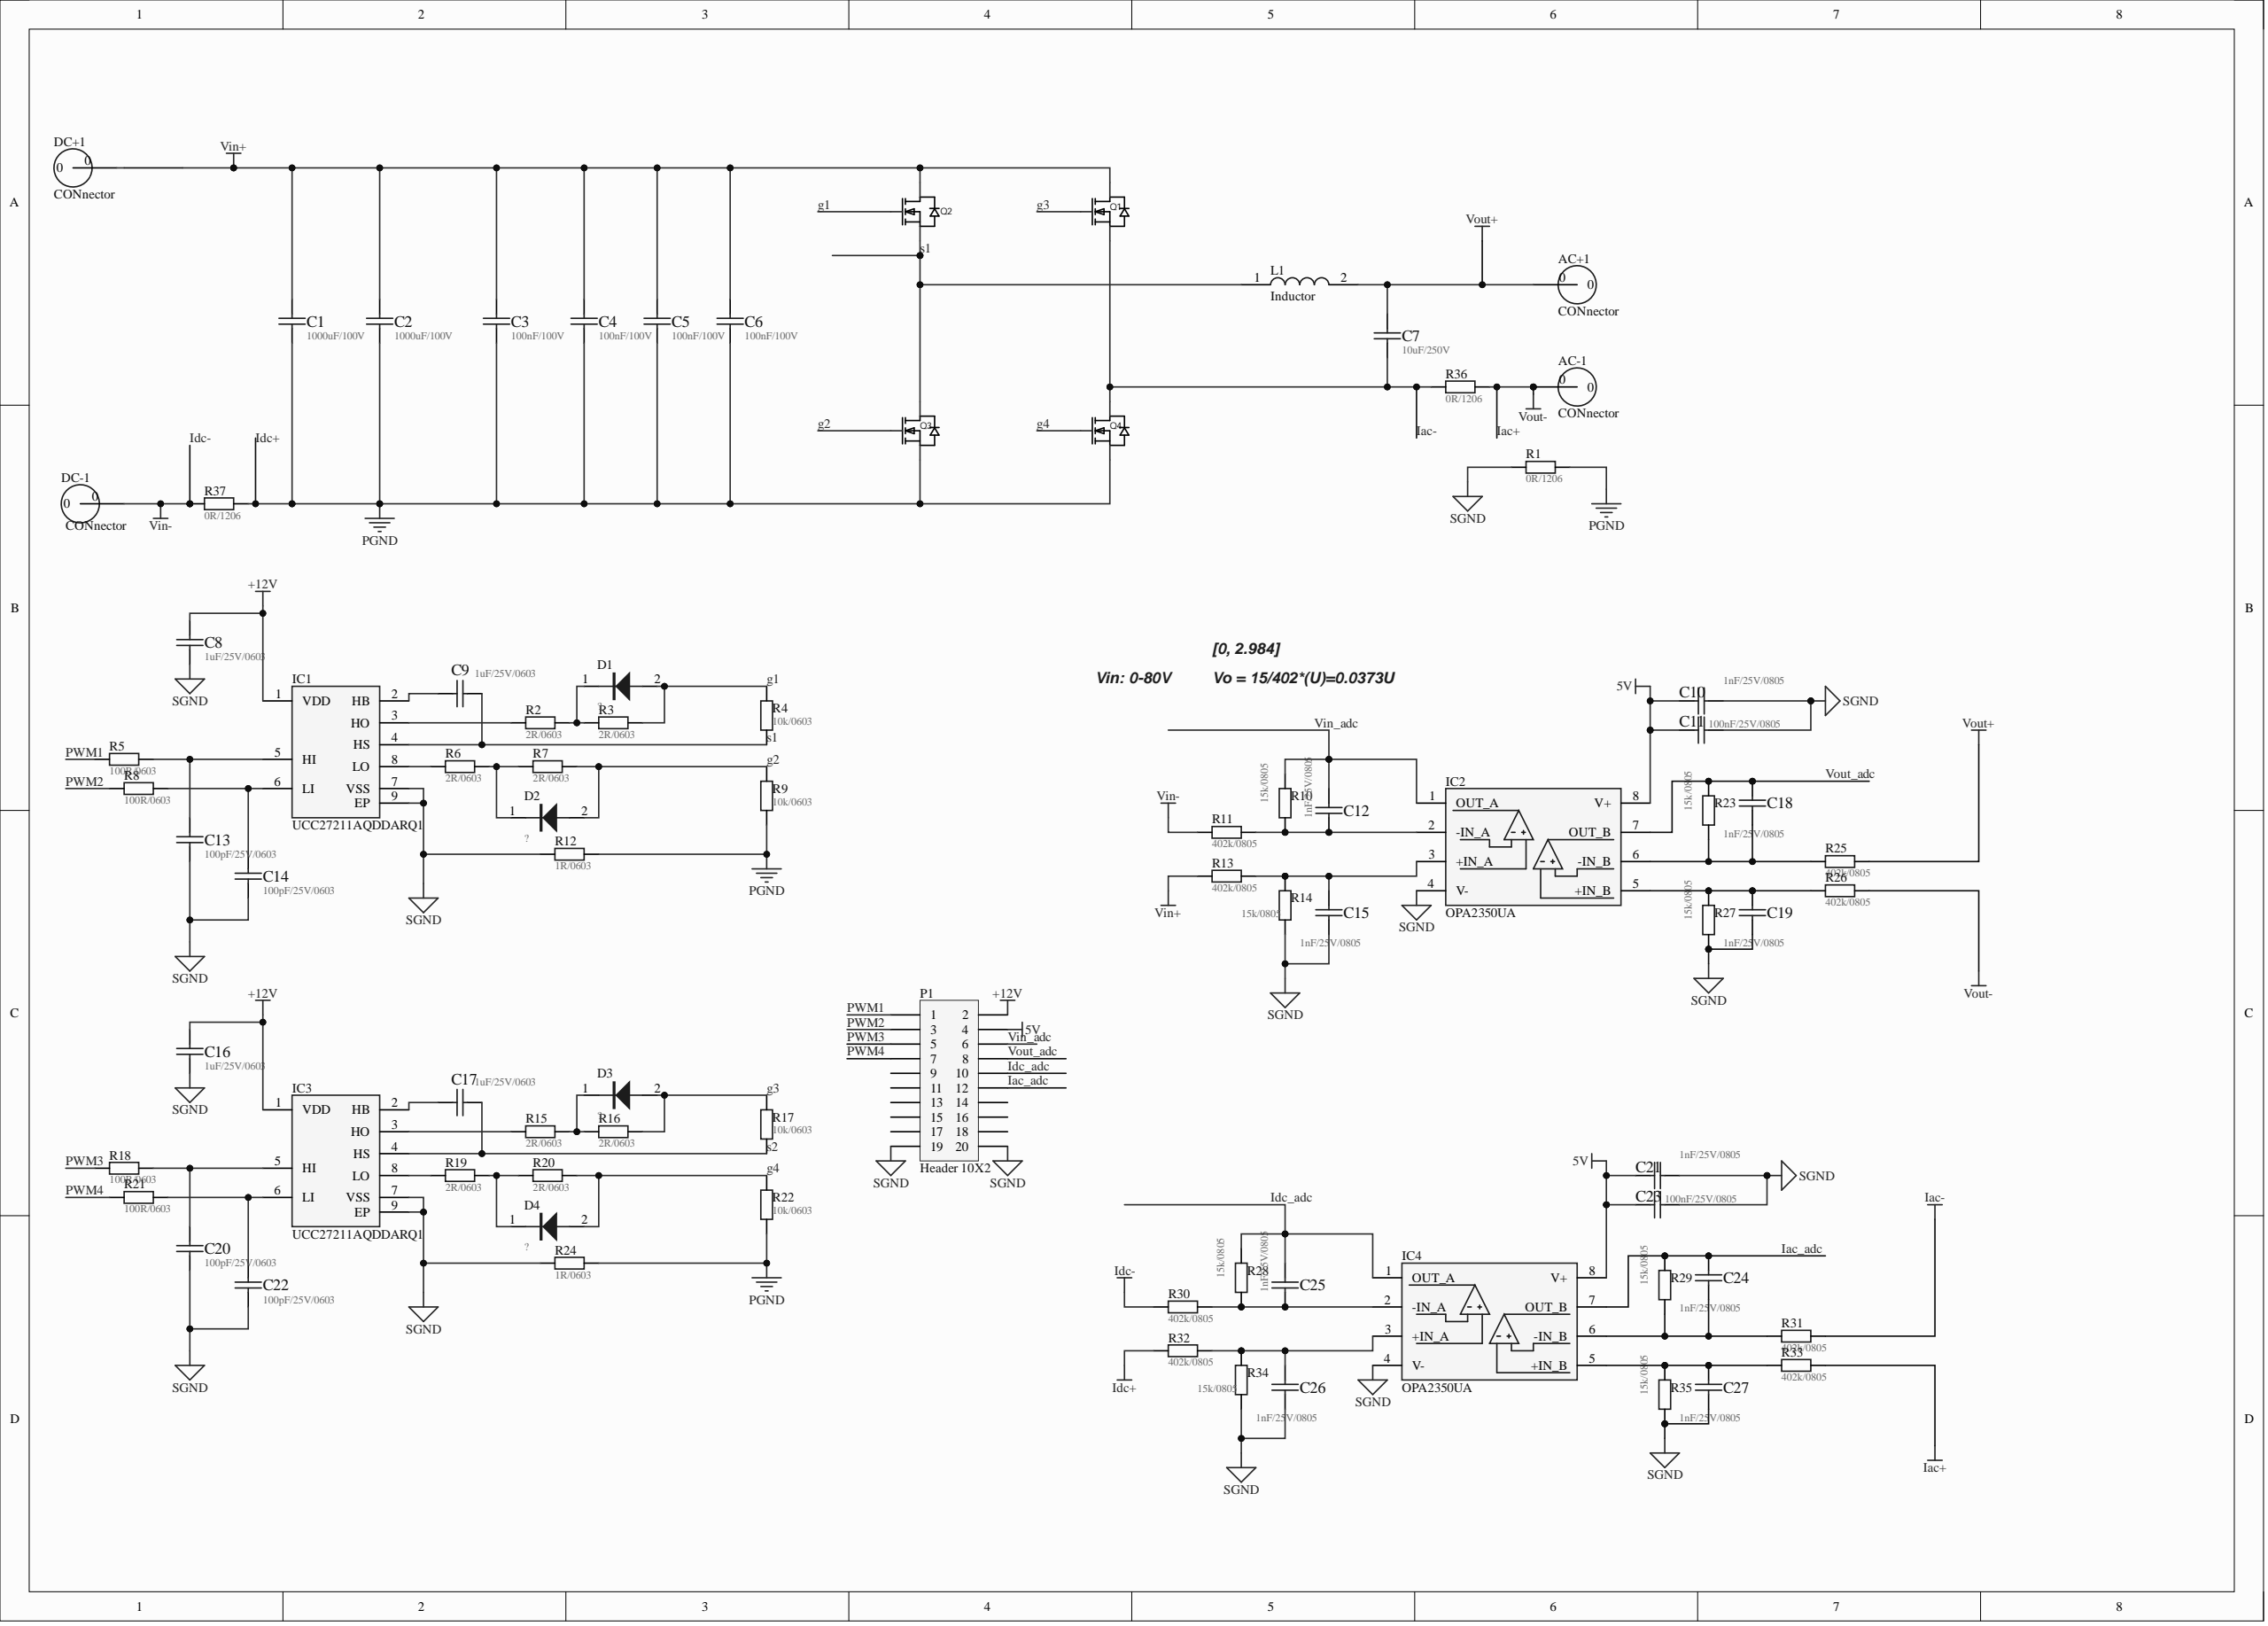Circuit board | Altium Designer | 82 parts | 45 nets
Bill of materials:
Comment,Description,Designator,Footprint,LibRef,Quantity
"CONnector","","AC-1, AC+1, DC-1, DC+1","CONN-TH_T44001","CONnector","4"
"1000uF/100V","","C1, C2","CAPE","CAP","2"
"100nF/100V","","C3, C4, C5, C6","0805C","CAP","4"
"10uF/250V","","C7","0805C","CAP","1"
"1uF/25V/0603","","C8, C9, C16, C17","0805C","CAP","4"
"1nF/25V/0805","","C10, C12, C15, C18, C19, C21, C24, C25, C26, C27","0805C","CAP","10"
"100nF/25V/0805","","C11, C23","0805C","CAP","2"
"100pF/25V/0603","","C13, C14, C20, C22","0805C","CAP","4"
"?","","D1, D2, D3, D4","SOD-323","DIODE_1","4"
"UCC27211AQDDARQ1","Integrated Circuit","IC1, IC3","SOIC8 Powerpad","UCC27211AQDDARQ1","2"
"OPA2350UA","Integrated Circuit","IC2, IC4","SOIC127P600X175-8N","OPA2350UA","2"
"Inductor","Inductor","L1","IND-TH_L55.0-W28.0-P20.00-D1.3","Inductor","1"
"Header 10X2","Header, 10-Pin, Dual row","P1","HDR2X10","Header 10X2","1"
"IPW60R037CSFD","","Q1, Q2, Q3, Q4","TO-247-3_L15.9-W5.1-P5.44-L","IPW60R037CSFD","4"
"0R/1206","Resistor","R1, R36, R37","0805R","Resistor","3"
"2R/0603","Resistor","R2, R3, R6, R7, R15, R16, R19, R20","0805R","Resistor","8"
"10k/0603","Resistor","R4, R9, R17, R22","0805R","Resistor","4"
"100R/0603","Resistor","R5, R8, R18, R21","0805R","Resistor","4"
"15k/0805","Resistor","R10, R14, R23, R27, R28, R29, R34, R35","0805R","Resistor","8"
"402k/0805","Resistor","R11, R13, R25, R26, R30, R31, R32, R33","0805R","Resistor","8"
"1R/0603","Resistor","R12, R24","0805R","Resistor","2"
Netlist (Protel format):
[
AC+1
CONN-TH_T44001
CONnector



]
[
AC-1
CONN-TH_T44001
CONnector



]
[
C1
CAPE
1000uF/100V



]
[
C2
CAPE
1000uF/100V



]
[
C3
0805C
100nF/100V



]
[
C4
0805C
100nF/100V



]
[
C5
0805C
100nF/100V



]
[
C6
0805C
100nF/100V



]
[
C7
0805C
10uF/250V



]
[
C8
0805C
1uF/25V/0603



]
[
C9
0805C
1uF/25V/0603



]
[
C10
0805C
1nF/25V/0805



]
[
C11
0805C
100nF/25V/0805



]
[
C12
0805C
1nF/25V/0805



]
[
C13
0805C
100pF/25V/0603



]
[
C14
0805C
100pF/25V/0603



]
[
C15
0805C
1nF/25V/0805



]
[
C16
0805C
1uF/25V/0603



]
[
C17
0805C
1uF/25V/0603



]
[
C18
0805C
1nF/25V/0805



]
[
C19
0805C
1nF/25V/0805



]
[
C20
0805C
100pF/25V/0603



]
[
C21
0805C
1nF/25V/0805



]
[
C22
0805C
100pF/25V/0603



]
[
C23
0805C
100nF/25V/0805



]
[
C24
0805C
1nF/25V/0805



]
[
C25
0805C
1nF/25V/0805



]
[
C26
0805C
1nF/25V/0805



]
[
C27
0805C
1nF/25V/0805



]
[
D1
SOD-323
?



]
[
D2
SOD-323
?



]
[
D3
SOD-323
?



]
[
D4
SOD-323
?



]
[
DC+1
CONN-TH_T44001
CONnector



]
[
DC-1
CONN-TH_T44001
CONnector



]
[
IC1
SOIC8 Powerpad
UCC27211AQDDARQ1



]
[
IC2
SOIC127P600X175-8N
OPA2350UA



]
[
IC3
SOIC8 Powerpad
UCC27211AQDDARQ1



]
[
IC4
SOIC127P600X175-8N
OPA2350UA



]
[
L1
IND-TH_L55.0-W28.0-P20.00-D1.3
Inductor



]
[
P1
HDR2X10
Header 10X2



]
[
Q1
TO-247-3_L15.9-W5.1-P5.44-L
IPW60R037CSFD



]
[
Q2
TO-247-3_L15.9-W5.1-P5.44-L
IPW60R037CSFD



]
[
Q3
TO-247-3_L15.9-W5.1-P5.44-L
IPW60R037CSFD



]
[
Q4
TO-247-3_L15.9-W5.1-P5.44-L
IPW60R037CSFD



]
[
R1
0805R
0R/1206



]
[
R2
0805R
2R/0603



]
[
R3
0805R
2R/0603



]
[
R4
0805R
10k/0603



]
[
R5
0805R
100R/0603



]
[
R6
0805R
2R/0603



]
[
R7
0805R
2R/0603



]
[
R8
0805R
100R/0603



]
[
R9
0805R
10k/0603



]
[
R10
0805R
15k/0805



]
[
R11
0805R
402k/0805



]
[
R12
0805R
1R/0603



]
[
R13
0805R
402k/0805



]
[
R14
0805R
15k/0805



]
[
R15
0805R
2R/0603



]
[
R16
0805R
2R/0603



]
[
R17
0805R
10k/0603



]
[
R18
0805R
100R/0603



]
[
R19
0805R
2R/0603



]
[
R20
0805R
2R/0603



]
[
R21
0805R
100R/0603



]
[
R22
0805R
10k/0603



]
[
R23
0805R
15k/0805



]
[
R24
0805R
1R/0603



]
[
R25
0805R
402k/0805



]
[
R26
0805R
402k/0805



]
[
R27
0805R
15k/0805



]
[
R28
0805R
15k/0805



]
[
R29
0805R
15k/0805



]
[
R30
0805R
402k/0805



]
[
R31
0805R
402k/0805



]
[
R32
0805R
402k/0805



]
[
R33
0805R
402k/0805



]
[
R34
0805R
15k/0805



]
[
R35
0805R
15k/0805



]
[
R36
0805R
0R/1206



]
[
R37
0805R
0R/1206



]
(
Vout_adc
C18-1
IC2-7
P1-8
R23-2
)
(
Vout+
AC+1-0
C7-1
L1-2
R25-2
)
(
Vin_adc
C12-1
IC2-1
P1-6
R10-2
)
(
Vin+
C1-1
C2-1
C3-1
C4-1
C5-1
C6-1
DC+1-0
Q1-2
Q2-2
R13-1
)
(
SGND
C8-1
C10-1
C11-1
C13-2
C14-2
C15-2
C16-1
C19-2
C20-2
C21-1
C22-2
C23-1
C26-2
C27-2
IC1-7
IC1-9
IC2-4
IC3-7
IC3-9
IC4-4
P1-19
P1-20
R1-2
R12-1
R14-1
R24-1
R27-1
R34-1
R35-1
)
(
s2
C17-2
IC3-4
R17-1
)
(
s1
C9-2
IC1-4
L1-1
Q2-3
Q3-2
R4-1
)
(
PWM4
P1-7
R21-1
)
(
PWM3
P1-5
R18-1
)
(
PWM2
P1-3
R8-1
)
(
PWM1
P1-1
R5-1
)
(
NetIC3_8
IC3-8
R19-1
)
(
NetIC3_3
IC3-3
R15-1
)
(
NetIC1_8
IC1-8
R6-1
)
(
NetIC1_3
IC1-3
R2-1
)
(
NetD4_1
D4-1
R19-2
R20-1
)
(
NetD3_1
D3-1
R15-2
R16-1
)
(
NetD2_1
D2-1
R6-2
R7-1
)
(
NetD1_1
D1-1
R2-2
R3-1
)
(
NetC27_1
C27-1
IC4-5
R33-1
R35-2
)
(
NetC26_1
C26-1
IC4-3
R32-2
R34-2
)
(
NetC25_2
C25-2
IC4-2
R28-1
R30-2
)
(
NetC24_2
C24-2
IC4-6
R29-1
R31-1
)
(
NetC22_1
C22-1
IC3-6
R21-2
)
(
NetC20_1
C20-1
IC3-5
R18-2
)
(
NetC19_1
C19-1
IC2-5
R26-1
R27-2
)
(
NetC18_2
C18-2
IC2-6
R23-1
R25-1
)
(
NetC17_1
C17-1
IC3-2
)
(
NetC15_1
C15-1
IC2-3
R13-2
R14-2
)
(
NetC14_1
C14-1
IC1-6
R8-2
)
(
NetC13_1
C13-1
IC1-5
R5-2
)
(
NetC12_2
C12-2
IC2-2
R10-1
R11-2
)
(
NetC9_1
C9-1
IC1-2
)
(
Idc_adc
C25-1
IC4-1
P1-10
R28-2
)
(
Idc-
DC-1-0
R11-1
R30-1
R37-2
)
(
Idc+
C1-2
C2-2
C3-2
C4-2
C5-2
C6-2
Q3-3
Q4-3
R1-1
R9-1
R12-2
R22-1
R24-2
R32-1
R37-1
)
(
Iac_adc
C24-1
IC4-7
P1-12
R29-2
)
(
Iac-
C7-2
Q1-3
Q4-2
R31-2
R36-2
)
(
Iac+
AC-1-0
R26-2
R33-2
R36-1
)
(
g4
D4-2
Q4-1
R20-2
R22-2
)
(
g3
D3-2
Q1-1
R16-2
R17-2
)
(
g2
D2-2
Q3-1
R7-2
R9-2
)
(
g1
D1-2
Q2-1
R3-2
R4-2
)
(
+12V
C8-2
C16-2
IC1-1
IC3-1
P1-2
)
(
5V
C10-2
C11-2
C21-2
C23-2
IC2-8
IC4-8
P1-4
)